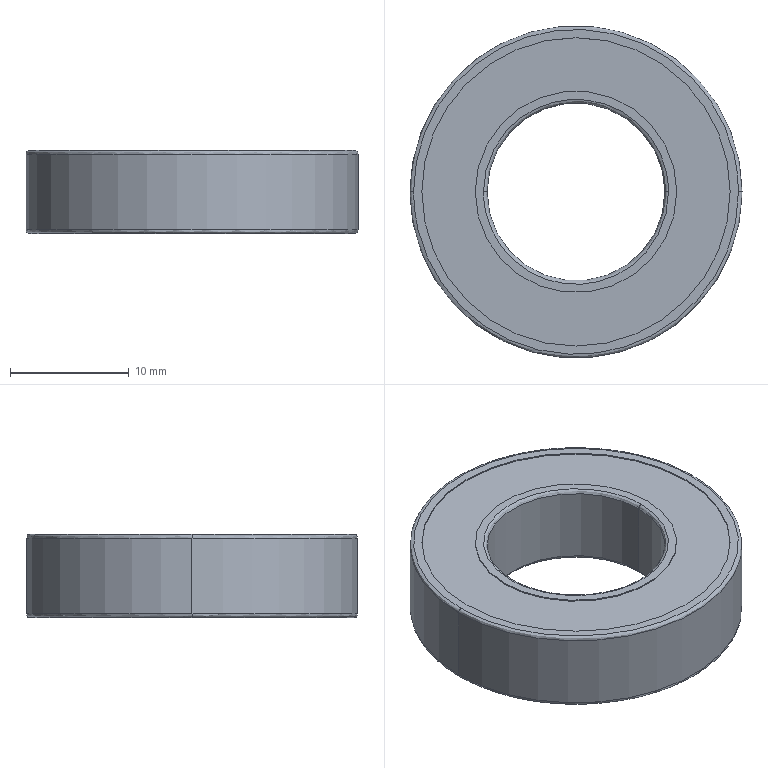Part | SolidWorks | features BaseBody 1 | 1 solid | 26 faces | box 28 x 28 x 7 mm | volume 3008 mm3 | cylinder 12 | spline 8 | plane 6 | commonest cylinder face diameters 17 x4 26 x4 15 x2 28 x2
STEP:
#1=CARTESIAN_POINT('',(-13.7,0.,-7.));
#2=VERTEX_POINT('',#1);
#3=CARTESIAN_POINT('',(13.7,0.,-7.));
#4=VERTEX_POINT('',#3);
#5=CARTESIAN_POINT('',(-13.7,0.,-7.));
#6=CARTESIAN_POINT('',(-13.7,-27.4,-7.));
#7=CARTESIAN_POINT('',(13.7,-27.4,-7.));
#8=CARTESIAN_POINT('',(13.7,0.,-7.));
#9=(BOUNDED_CURVE()B_SPLINE_CURVE(3,(#5,#6,#7,#8),.UNSPECIFIED.,.F.,.F.)B_SPLINE_CURVE_WITH_KNOTS((4,4),(0.,0.5),.UNSPECIFIED.)CURVE()GEOMETRIC_REPRESENTATION_ITEM()RATIONAL_B_SPLINE_CURVE((1.,0.3333,0.3333,1.))REPRESENTATION_ITEM(''));
#10=EDGE_CURVE('',#2,#4,#9,.T.);
#11=ORIENTED_EDGE('',*,*,#10,.T.);
#12=CARTESIAN_POINT('',(14.,0.,-6.7));
#13=VERTEX_POINT('',#12);
#14=CARTESIAN_POINT('',(13.7,0.,-6.7));
#15=DIRECTION('',(0.,-1.,0.));
#16=DIRECTION('',(1.,0.,0.));
#17=AXIS2_PLACEMENT_3D('',#14,#15,#16);
#18=CIRCLE('',#17,0.3);
#19=EDGE_CURVE('',#4,#13,#18,.T.);
#20=ORIENTED_EDGE('',*,*,#19,.T.);
#21=CARTESIAN_POINT('',(-14.,0.,-6.7));
#22=VERTEX_POINT('',#21);
#23=CARTESIAN_POINT('',(0.,0.,-6.7));
#24=DIRECTION('',(0.,0.,1.));
#25=DIRECTION('',(1.,0.,0.));
#26=AXIS2_PLACEMENT_3D('',#23,#24,#25);
#27=CIRCLE('',#26,14.);
#28=EDGE_CURVE('',#22,#13,#27,.T.);
#29=ORIENTED_EDGE('',*,*,#28,.F.);
#30=CARTESIAN_POINT('',(-13.7,0.,-6.7));
#31=DIRECTION('',(0.,1.,0.));
#32=DIRECTION('',(-1.,0.,0.));
#33=AXIS2_PLACEMENT_3D('',#30,#31,#32);
#34=CIRCLE('',#33,0.3);
#35=EDGE_CURVE('',#2,#22,#34,.T.);
#36=ORIENTED_EDGE('',*,*,#35,.F.);
#37=EDGE_LOOP('',(#11,#20,#29,#36));
#38=FACE_OUTER_BOUND('',#37,.T.);
#39=CARTESIAN_POINT('',(13.7,0.,-7.));
#40=CARTESIAN_POINT('',(13.7,-27.4,-7.));
#41=CARTESIAN_POINT('',(-13.7,-27.4,-7.));
#42=CARTESIAN_POINT('',(-13.7,0.,-7.));
#43=CARTESIAN_POINT('',(13.876,0.,-7.));
#44=CARTESIAN_POINT('',(13.876,-27.751,-7.));
#45=CARTESIAN_POINT('',(-13.876,-27.751,-7.));
#46=CARTESIAN_POINT('',(-13.876,0.,-7.));
#47=CARTESIAN_POINT('',(14.,0.,-6.876));
#48=CARTESIAN_POINT('',(14.,-28.,-6.876));
#49=CARTESIAN_POINT('',(-14.,-28.,-6.876));
#50=CARTESIAN_POINT('',(-14.,0.,-6.876));
#51=CARTESIAN_POINT('',(14.,0.,-6.7));
#52=CARTESIAN_POINT('',(14.,-28.,-6.7));
#53=CARTESIAN_POINT('',(-14.,-28.,-6.7));
#54=CARTESIAN_POINT('',(-14.,0.,-6.7));
#55=(BOUNDED_SURFACE()B_SPLINE_SURFACE(3,3,((#39,#40,#41,#42),(#43,#44,#45,#46),(#47,#48,#49,#50),(#51,#52,#53,#54)),.UNSPECIFIED.,.F.,.F.,.F.)B_SPLINE_SURFACE_WITH_KNOTS((4,4),(4,4),(0.,1.),(0.,1.),.UNSPECIFIED.)GEOMETRIC_REPRESENTATION_ITEM()RATIONAL_B_SPLINE_SURFACE(((1.,0.3333,0.3333,1.),(0.8047,0.2682,0.2682,0.8047),(0.8047,0.2682,0.2682,0.8047),(1.,0.3333,0.3333,1.)))REPRESENTATION_ITEM('')SURFACE());
#56=ADVANCED_FACE('',(#38),#55,.T.);
#57=CARTESIAN_POINT('',(14.,0.,-0.3));
#58=VERTEX_POINT('',#57);
#59=CARTESIAN_POINT('',(-14.,0.,-0.3));
#60=VERTEX_POINT('',#59);
#61=CARTESIAN_POINT('',(0.,0.,-0.3));
#62=DIRECTION('',(0.,0.,-1.));
#63=DIRECTION('',(1.,0.,0.));
#64=AXIS2_PLACEMENT_3D('',#61,#62,#63);
#65=CIRCLE('',#64,14.);
#66=EDGE_CURVE('',#58,#60,#65,.T.);
#67=ORIENTED_EDGE('',*,*,#66,.F.);
#68=CARTESIAN_POINT('',(13.7,0.,0.));
#69=VERTEX_POINT('',#68);
#70=CARTESIAN_POINT('',(13.7,0.,-0.3));
#71=DIRECTION('',(0.,-1.,0.));
#72=DIRECTION('',(1.,0.,0.));
#73=AXIS2_PLACEMENT_3D('',#70,#71,#72);
#74=CIRCLE('',#73,0.3);
#75=EDGE_CURVE('',#58,#69,#74,.T.);
#76=ORIENTED_EDGE('',*,*,#75,.T.);
#77=CARTESIAN_POINT('',(-13.7,0.,0.));
#78=VERTEX_POINT('',#77);
#79=CARTESIAN_POINT('',(13.7,0.,0.));
#80=CARTESIAN_POINT('',(13.7,-27.4,0.));
#81=CARTESIAN_POINT('',(-13.7,-27.4,0.));
#82=CARTESIAN_POINT('',(-13.7,0.,0.));
#83=(BOUNDED_CURVE()B_SPLINE_CURVE(3,(#79,#80,#81,#82),.UNSPECIFIED.,.F.,.F.)B_SPLINE_CURVE_WITH_KNOTS((4,4),(0.5,1.),.UNSPECIFIED.)CURVE()GEOMETRIC_REPRESENTATION_ITEM()RATIONAL_B_SPLINE_CURVE((1.,0.3333,0.3333,1.))REPRESENTATION_ITEM(''));
#84=EDGE_CURVE('',#69,#78,#83,.T.);
#85=ORIENTED_EDGE('',*,*,#84,.T.);
#86=CARTESIAN_POINT('',(-13.7,0.,-0.3));
#87=DIRECTION('',(0.,1.,0.));
#88=DIRECTION('',(-1.,0.,0.));
#89=AXIS2_PLACEMENT_3D('',#86,#87,#88);
#90=CIRCLE('',#89,0.3);
#91=EDGE_CURVE('',#60,#78,#90,.T.);
#92=ORIENTED_EDGE('',*,*,#91,.F.);
#93=EDGE_LOOP('',(#67,#76,#85,#92));
#94=FACE_OUTER_BOUND('',#93,.T.);
#95=CARTESIAN_POINT('',(14.,0.,-0.3));
#96=CARTESIAN_POINT('',(14.,-28.,-0.3));
#97=CARTESIAN_POINT('',(-14.,-28.,-0.3));
#98=CARTESIAN_POINT('',(-14.,0.,-0.3));
#99=CARTESIAN_POINT('',(14.,0.,-0.1243));
#100=CARTESIAN_POINT('',(14.,-28.,-0.1243));
#101=CARTESIAN_POINT('',(-14.,-28.,-0.1243));
#102=CARTESIAN_POINT('',(-14.,0.,-0.1243));
#103=CARTESIAN_POINT('',(13.876,0.,0.));
#104=CARTESIAN_POINT('',(13.876,-27.751,0.));
#105=CARTESIAN_POINT('',(-13.876,-27.751,0.));
#106=CARTESIAN_POINT('',(-13.876,0.,0.));
#107=CARTESIAN_POINT('',(13.7,0.,0.));
#108=CARTESIAN_POINT('',(13.7,-27.4,0.));
#109=CARTESIAN_POINT('',(-13.7,-27.4,0.));
#110=CARTESIAN_POINT('',(-13.7,0.,0.));
#111=(BOUNDED_SURFACE()B_SPLINE_SURFACE(3,3,((#95,#96,#97,#98),(#99,#100,#101,#102),(#103,#104,#105,#106),(#107,#108,#109,#110)),.UNSPECIFIED.,.F.,.F.,.F.)B_SPLINE_SURFACE_WITH_KNOTS((4,4),(4,4),(0.,1.),(0.,1.),.UNSPECIFIED.)GEOMETRIC_REPRESENTATION_ITEM()RATIONAL_B_SPLINE_SURFACE(((1.,0.3333,0.3333,1.),(0.8047,0.2682,0.2682,0.8047),(0.8047,0.2682,0.2682,0.8047),(1.,0.3333,0.3333,1.)))REPRESENTATION_ITEM('')SURFACE());
#112=ADVANCED_FACE('',(#94),#111,.T.);
#113=CARTESIAN_POINT('',(-7.5,0.,-6.7));
#114=VERTEX_POINT('',#113);
#115=CARTESIAN_POINT('',(7.5,0.,-6.7));
#116=VERTEX_POINT('',#115);
#117=CARTESIAN_POINT('',(0.,0.,-6.7));
#118=DIRECTION('',(0.,0.,1.));
#119=DIRECTION('',(-1.,0.,0.));
#120=AXIS2_PLACEMENT_3D('',#117,#118,#119);
#121=CIRCLE('',#120,7.5);
#122=EDGE_CURVE('',#114,#116,#121,.T.);
#123=ORIENTED_EDGE('',*,*,#122,.T.);
#124=CARTESIAN_POINT('',(7.8,0.,-7.));
#125=VERTEX_POINT('',#124);
#126=CARTESIAN_POINT('',(7.8,0.,-6.7));
#127=DIRECTION('',(0.,-1.,0.));
#128=DIRECTION('',(1.,0.,0.));
#129=AXIS2_PLACEMENT_3D('',#126,#127,#128);
#130=CIRCLE('',#129,0.3);
#131=EDGE_CURVE('',#116,#125,#130,.T.);
#132=ORIENTED_EDGE('',*,*,#131,.T.);
#133=CARTESIAN_POINT('',(-7.8,0.,-7.));
#134=VERTEX_POINT('',#133);
#135=CARTESIAN_POINT('',(-7.8,0.,-7.));
#136=CARTESIAN_POINT('',(-7.8,-0.2385,-7.));
#137=CARTESIAN_POINT('',(-7.784,-0.5947,-7.));
#138=CARTESIAN_POINT('',(-7.736,-1.008,-7.));
#139=CARTESIAN_POINT('',(-7.705,-1.214,-7.));
#140=CARTESIAN_POINT('',(-7.691,-1.302,-7.));
#141=CARTESIAN_POINT('',(-7.68,-1.361,-7.));
#142=CARTESIAN_POINT('',(-7.676,-1.388,-7.));
#143=CARTESIAN_POINT('',(-7.624,-1.668,-7.));
#144=CARTESIAN_POINT('',(-7.537,-2.036,-7.));
#145=CARTESIAN_POINT('',(-7.405,-2.456,-7.));
#146=CARTESIAN_POINT('',(-7.331,-2.664,-7.));
#147=CARTESIAN_POINT('',(-7.298,-2.753,-7.));
#148=CARTESIAN_POINT('',(-7.275,-2.812,-7.));
#149=CARTESIAN_POINT('',(-7.264,-2.841,-7.));
#150=CARTESIAN_POINT('',(-7.155,-3.116,-7.));
#151=CARTESIAN_POINT('',(-6.992,-3.474,-7.));
#152=CARTESIAN_POINT('',(-6.771,-3.877,-7.));
#153=CARTESIAN_POINT('',(-6.669,-4.046,-7.));
#154=CARTESIAN_POINT('',(-6.6,-4.157,-7.));
#155=CARTESIAN_POINT('',(-6.565,-4.212,-7.));
#156=CARTESIAN_POINT('',(-6.234,-4.719,-7.));
#157=CARTESIAN_POINT('',(-5.896,-5.135,-7.));
#158=CARTESIAN_POINT('',(-5.325,-5.706,-7.));
#159=CARTESIAN_POINT('',(-5.027,-5.975,-7.));
#160=CARTESIAN_POINT('',(-4.655,-6.261,-7.));
#161=CARTESIAN_POINT('',(-4.491,-6.378,-7.));
#162=CARTESIAN_POINT('',(-4.38,-6.454,-7.));
#163=CARTESIAN_POINT('',(-4.323,-6.493,-7.));
#164=CARTESIAN_POINT('',(-4.048,-6.673,-7.));
#165=CARTESIAN_POINT('',(-3.708,-6.871,-7.));
#166=CARTESIAN_POINT('',(-3.295,-7.072,-7.));
#167=CARTESIAN_POINT('',(-3.084,-7.165,-7.));
#168=CARTESIAN_POINT('',(-2.993,-7.203,-7.));
#169=CARTESIAN_POINT('',(-2.932,-7.228,-7.));
#170=CARTESIAN_POINT('',(-2.901,-7.241,-7.));
#171=CARTESIAN_POINT('',(-2.636,-7.345,-7.));
#172=CARTESIAN_POINT('',(-2.278,-7.467,-7.));
#173=CARTESIAN_POINT('',(-1.852,-7.579,-7.));
#174=CARTESIAN_POINT('',(-1.636,-7.627,-7.));
#175=CARTESIAN_POINT('',(-1.543,-7.646,-7.));
#176=CARTESIAN_POINT('',(-1.481,-7.658,-7.));
#177=CARTESIAN_POINT('',(-1.449,-7.664,-7.));
#178=CARTESIAN_POINT('',(-0.9505,-7.757,-7.));
#179=CARTESIAN_POINT('',(-0.4767,-7.8,-7.));
#180=CARTESIAN_POINT('',(0.2384,-7.8,-7.));
#181=CARTESIAN_POINT('',(0.5946,-7.784,-7.));
#182=CARTESIAN_POINT('',(1.008,-7.736,-7.));
#183=CARTESIAN_POINT('',(1.214,-7.705,-7.));
#184=CARTESIAN_POINT('',(1.302,-7.691,-7.));
#185=CARTESIAN_POINT('',(1.361,-7.68,-7.));
#186=CARTESIAN_POINT('',(1.388,-7.676,-7.));
#187=CARTESIAN_POINT('',(1.668,-7.624,-7.));
#188=CARTESIAN_POINT('',(2.036,-7.537,-7.));
#189=CARTESIAN_POINT('',(2.456,-7.405,-7.));
#190=CARTESIAN_POINT('',(2.664,-7.331,-7.));
#191=CARTESIAN_POINT('',(2.753,-7.298,-7.));
#192=CARTESIAN_POINT('',(2.812,-7.275,-7.));
#193=CARTESIAN_POINT('',(2.841,-7.264,-7.));
#194=CARTESIAN_POINT('',(3.116,-7.155,-7.));
#195=CARTESIAN_POINT('',(3.474,-6.992,-7.));
#196=CARTESIAN_POINT('',(3.877,-6.771,-7.));
#197=CARTESIAN_POINT('',(4.046,-6.669,-7.));
#198=CARTESIAN_POINT('',(4.157,-6.6,-7.));
#199=CARTESIAN_POINT('',(4.212,-6.565,-7.));
#200=CARTESIAN_POINT('',(4.719,-6.234,-7.));
#201=CARTESIAN_POINT('',(5.135,-5.896,-7.));
#202=CARTESIAN_POINT('',(5.706,-5.325,-7.));
#203=CARTESIAN_POINT('',(5.975,-5.027,-7.));
#204=CARTESIAN_POINT('',(6.261,-4.655,-7.));
#205=CARTESIAN_POINT('',(6.378,-4.491,-7.));
#206=CARTESIAN_POINT('',(6.454,-4.38,-7.));
#207=CARTESIAN_POINT('',(6.493,-4.323,-7.));
#208=CARTESIAN_POINT('',(6.673,-4.048,-7.));
#209=CARTESIAN_POINT('',(6.871,-3.708,-7.));
#210=CARTESIAN_POINT('',(7.072,-3.295,-7.));
#211=CARTESIAN_POINT('',(7.165,-3.084,-7.));
#212=CARTESIAN_POINT('',(7.203,-2.993,-7.));
#213=CARTESIAN_POINT('',(7.228,-2.932,-7.));
#214=CARTESIAN_POINT('',(7.241,-2.901,-7.));
#215=CARTESIAN_POINT('',(7.345,-2.636,-7.));
#216=CARTESIAN_POINT('',(7.467,-2.278,-7.));
#217=CARTESIAN_POINT('',(7.579,-1.852,-7.));
#218=CARTESIAN_POINT('',(7.627,-1.636,-7.));
#219=CARTESIAN_POINT('',(7.646,-1.543,-7.));
#220=CARTESIAN_POINT('',(7.658,-1.481,-7.));
#221=CARTESIAN_POINT('',(7.664,-1.449,-7.));
#222=CARTESIAN_POINT('',(7.757,-0.9505,-7.));
#223=CARTESIAN_POINT('',(7.8,-0.4767,-7.));
#224=CARTESIAN_POINT('',(7.8,0.,-7.));
#225=B_SPLINE_CURVE_WITH_KNOTS('',3,(#135,#136,#137,#138,#139,#140,#141,#142,#143,#144,#145,#146,#147,#148,#149,#150,#151,#152,#153,#154,#155,#156,#157,#158,#159,#160,#161,#162,#163,#164,#165,#166,#167,#168,#169,#170,#171,#172,#173,#174,#175,#176,#177,#178,#179,#180,#181,#182,#183,#184,#185,#186,#187,#188,#189,#190,#191,#192,#193,#194,#195,#196,#197,#198,#199,#200,#201,#202,#203,#204,#205,#206,#207,#208,#209,#210,#211,#212,#213,#214,#215,#216,#217,#218,#219,#220,#221,#222,#223,#224),.UNSPECIFIED.,.F.,.F.,(4,1,1,1,2,2,1,1,1,2,2,1,1,2,2,2,1,1,2,2,1,1,1,2,2,1,1,1,2,2,2,1,1,1,2,2,1,1,1,2,2,1,1,2,2,2,1,1,2,2,1,1,1,2,2,1,1,1,2,2,4),(0.,0.01562,0.02344,0.02734,0.0293,0.03125,0.04687,0.05469,0.05859,0.06055,0.0625,0.07812,0.08594,0.08984,0.09375,0.125,0.1406,0.1484,0.1523,0.1562,0.1719,0.1797,0.1836,0.1855,0.1875,0.2031,0.2109,0.2148,0.2168,0.2187,0.25,0.2656,0.2734,0.2773,0.2793,0.2812,0.2969,0.3047,0.3086,0.3105,0.3125,0.3281,0.3359,0.3398,0.3437,0.375,0.3906,0.3984,0.4023,0.4062,0.4219,0.4297,0.4336,0.4355,0.4375,0.4531,0.4609,0.4648,0.4668,0.4687,0.5),.UNSPECIFIED.);
#226=EDGE_CURVE('',#134,#125,#225,.T.);
#227=ORIENTED_EDGE('',*,*,#226,.F.);
#228=CARTESIAN_POINT('',(-7.8,0.,-6.7));
#229=DIRECTION('',(0.,1.,0.));
#230=DIRECTION('',(-1.,0.,0.));
#231=AXIS2_PLACEMENT_3D('',#228,#229,#230);
#232=CIRCLE('',#231,0.3);
#233=EDGE_CURVE('',#114,#134,#232,.T.);
#234=ORIENTED_EDGE('',*,*,#233,.F.);
#235=EDGE_LOOP('',(#123,#132,#227,#234));
#236=FACE_OUTER_BOUND('',#235,.T.);
#237=CARTESIAN_POINT('',(7.5,0.,-6.7));
#238=CARTESIAN_POINT('',(7.5,-15.,-6.7));
#239=CARTESIAN_POINT('',(-7.5,-15.,-6.7));
#240=CARTESIAN_POINT('',(-7.5,0.,-6.7));
#241=CARTESIAN_POINT('',(7.5,0.,-6.876));
#242=CARTESIAN_POINT('',(7.5,-15.,-6.876));
#243=CARTESIAN_POINT('',(-7.5,-15.,-6.876));
#244=CARTESIAN_POINT('',(-7.5,0.,-6.876));
#245=CARTESIAN_POINT('',(7.624,0.,-7.));
#246=CARTESIAN_POINT('',(7.624,-15.249,-7.));
#247=CARTESIAN_POINT('',(-7.624,-15.249,-7.));
#248=CARTESIAN_POINT('',(-7.624,0.,-7.));
#249=CARTESIAN_POINT('',(7.8,0.,-7.));
#250=CARTESIAN_POINT('',(7.8,-15.6,-7.));
#251=CARTESIAN_POINT('',(-7.8,-15.6,-7.));
#252=CARTESIAN_POINT('',(-7.8,0.,-7.));
#253=(BOUNDED_SURFACE()B_SPLINE_SURFACE(3,3,((#237,#238,#239,#240),(#241,#242,#243,#244),(#245,#246,#247,#248),(#249,#250,#251,#252)),.UNSPECIFIED.,.F.,.F.,.F.)B_SPLINE_SURFACE_WITH_KNOTS((4,4),(4,4),(0.,1.),(0.,1.),.UNSPECIFIED.)GEOMETRIC_REPRESENTATION_ITEM()RATIONAL_B_SPLINE_SURFACE(((1.,0.3333,0.3333,1.),(0.8047,0.2682,0.2682,0.8047),(0.8047,0.2682,0.2682,0.8047),(1.,0.3333,0.3333,1.)))REPRESENTATION_ITEM('')SURFACE());
#254=ADVANCED_FACE('',(#236),#253,.T.);
#255=CARTESIAN_POINT('',(7.8,0.,0.));
#256=VERTEX_POINT('',#255);
#257=CARTESIAN_POINT('',(-7.8,0.,0.));
#258=VERTEX_POINT('',#257);
#259=CARTESIAN_POINT('',(7.8,0.,0.));
#260=CARTESIAN_POINT('',(7.8,-0.2384,0.));
#261=CARTESIAN_POINT('',(7.784,-0.5946,0.));
#262=CARTESIAN_POINT('',(7.736,-1.008,0.));
#263=CARTESIAN_POINT('',(7.705,-1.214,0.));
#264=CARTESIAN_POINT('',(7.691,-1.302,0.));
#265=CARTESIAN_POINT('',(7.68,-1.361,0.));
#266=CARTESIAN_POINT('',(7.676,-1.388,0.));
#267=CARTESIAN_POINT('',(7.624,-1.668,0.));
#268=CARTESIAN_POINT('',(7.537,-2.036,0.));
#269=CARTESIAN_POINT('',(7.405,-2.456,0.));
#270=CARTESIAN_POINT('',(7.331,-2.664,0.));
#271=CARTESIAN_POINT('',(7.298,-2.753,0.));
#272=CARTESIAN_POINT('',(7.275,-2.812,0.));
#273=CARTESIAN_POINT('',(7.264,-2.841,0.));
#274=CARTESIAN_POINT('',(7.155,-3.116,0.));
#275=CARTESIAN_POINT('',(6.992,-3.474,0.));
#276=CARTESIAN_POINT('',(6.771,-3.877,0.));
#277=CARTESIAN_POINT('',(6.669,-4.046,0.));
#278=CARTESIAN_POINT('',(6.6,-4.157,0.));
#279=CARTESIAN_POINT('',(6.565,-4.212,0.));
#280=CARTESIAN_POINT('',(6.234,-4.719,0.));
#281=CARTESIAN_POINT('',(5.896,-5.135,0.));
#282=CARTESIAN_POINT('',(5.325,-5.706,0.));
#283=CARTESIAN_POINT('',(5.027,-5.975,0.));
#284=CARTESIAN_POINT('',(4.655,-6.261,0.));
#285=CARTESIAN_POINT('',(4.491,-6.378,0.));
#286=CARTESIAN_POINT('',(4.38,-6.454,0.));
#287=CARTESIAN_POINT('',(4.323,-6.493,0.));
#288=CARTESIAN_POINT('',(4.048,-6.673,0.));
#289=CARTESIAN_POINT('',(3.708,-6.871,0.));
#290=CARTESIAN_POINT('',(3.295,-7.072,0.));
#291=CARTESIAN_POINT('',(3.084,-7.165,0.));
#292=CARTESIAN_POINT('',(2.993,-7.203,0.));
#293=CARTESIAN_POINT('',(2.932,-7.228,0.));
#294=CARTESIAN_POINT('',(2.901,-7.241,0.));
#295=CARTESIAN_POINT('',(2.636,-7.345,0.));
#296=CARTESIAN_POINT('',(2.278,-7.467,0.));
#297=CARTESIAN_POINT('',(1.852,-7.579,0.));
#298=CARTESIAN_POINT('',(1.636,-7.627,0.));
#299=CARTESIAN_POINT('',(1.543,-7.646,0.));
#300=CARTESIAN_POINT('',(1.481,-7.658,0.));
#301=CARTESIAN_POINT('',(1.449,-7.664,0.));
#302=CARTESIAN_POINT('',(0.9505,-7.757,0.));
#303=CARTESIAN_POINT('',(0.4767,-7.8,0.));
#304=CARTESIAN_POINT('',(-0.2384,-7.8,0.));
#305=CARTESIAN_POINT('',(-0.5946,-7.784,0.));
#306=CARTESIAN_POINT('',(-1.008,-7.736,0.));
#307=CARTESIAN_POINT('',(-1.214,-7.705,0.));
#308=CARTESIAN_POINT('',(-1.302,-7.691,0.));
#309=CARTESIAN_POINT('',(-1.361,-7.68,0.));
#310=CARTESIAN_POINT('',(-1.388,-7.676,0.));
#311=CARTESIAN_POINT('',(-1.668,-7.624,0.));
#312=CARTESIAN_POINT('',(-2.036,-7.537,0.));
#313=CARTESIAN_POINT('',(-2.456,-7.405,0.));
#314=CARTESIAN_POINT('',(-2.664,-7.331,0.));
#315=CARTESIAN_POINT('',(-2.753,-7.298,0.));
#316=CARTESIAN_POINT('',(-2.812,-7.275,0.));
#317=CARTESIAN_POINT('',(-2.841,-7.264,0.));
#318=CARTESIAN_POINT('',(-3.116,-7.155,0.));
#319=CARTESIAN_POINT('',(-3.474,-6.992,0.));
#320=CARTESIAN_POINT('',(-3.877,-6.771,0.));
#321=CARTESIAN_POINT('',(-4.046,-6.669,0.));
#322=CARTESIAN_POINT('',(-4.157,-6.6,0.));
#323=CARTESIAN_POINT('',(-4.212,-6.565,0.));
#324=CARTESIAN_POINT('',(-4.719,-6.234,0.));
#325=CARTESIAN_POINT('',(-5.135,-5.896,0.));
#326=CARTESIAN_POINT('',(-5.706,-5.325,0.));
#327=CARTESIAN_POINT('',(-5.975,-5.027,0.));
#328=CARTESIAN_POINT('',(-6.261,-4.655,0.));
#329=CARTESIAN_POINT('',(-6.378,-4.491,0.));
#330=CARTESIAN_POINT('',(-6.454,-4.38,0.));
#331=CARTESIAN_POINT('',(-6.493,-4.323,0.));
#332=CARTESIAN_POINT('',(-6.673,-4.048,0.));
#333=CARTESIAN_POINT('',(-6.871,-3.708,0.));
#334=CARTESIAN_POINT('',(-7.072,-3.295,0.));
#335=CARTESIAN_POINT('',(-7.165,-3.084,0.));
#336=CARTESIAN_POINT('',(-7.203,-2.993,0.));
#337=CARTESIAN_POINT('',(-7.228,-2.932,0.));
#338=CARTESIAN_POINT('',(-7.241,-2.901,0.));
#339=CARTESIAN_POINT('',(-7.345,-2.636,0.));
#340=CARTESIAN_POINT('',(-7.467,-2.278,0.));
#341=CARTESIAN_POINT('',(-7.579,-1.852,0.));
#342=CARTESIAN_POINT('',(-7.627,-1.636,0.));
#343=CARTESIAN_POINT('',(-7.646,-1.543,0.));
#344=CARTESIAN_POINT('',(-7.658,-1.481,0.));
#345=CARTESIAN_POINT('',(-7.664,-1.449,0.));
#346=CARTESIAN_POINT('',(-7.757,-0.9504,0.));
#347=CARTESIAN_POINT('',(-7.8,-0.4773,0.));
#348=CARTESIAN_POINT('',(-7.8,0.,0.));
#349=B_SPLINE_CURVE_WITH_KNOTS('',3,(#259,#260,#261,#262,#263,#264,#265,#266,#267,#268,#269,#270,#271,#272,#273,#274,#275,#276,#277,#278,#279,#280,#281,#282,#283,#284,#285,#286,#287,#288,#289,#290,#291,#292,#293,#294,#295,#296,#297,#298,#299,#300,#301,#302,#303,#304,#305,#306,#307,#308,#309,#310,#311,#312,#313,#314,#315,#316,#317,#318,#319,#320,#321,#322,#323,#324,#325,#326,#327,#328,#329,#330,#331,#332,#333,#334,#335,#336,#337,#338,#339,#340,#341,#342,#343,#344,#345,#346,#347,#348),.UNSPECIFIED.,.F.,.F.,(4,1,1,1,2,2,1,1,1,2,2,1,1,2,2,2,1,1,2,2,1,1,1,2,2,1,1,1,2,2,2,1,1,1,2,2,1,1,1,2,2,1,1,2,2,2,1,1,2,2,1,1,1,2,2,1,1,1,2,2,4),(0.5,0.5156,0.5234,0.5273,0.5293,0.5313,0.5469,0.5547,0.5586,0.5605,0.5625,0.5781,0.5859,0.5898,0.5938,0.625,0.6406,0.6484,0.6523,0.6562,0.6719,0.6797,0.6836,0.6855,0.6875,0.7031,0.7109,0.7148,0.7168,0.7187,0.75,0.7656,0.7734,0.7773,0.7793,0.7812,0.7969,0.8047,0.8086,0.8105,0.8125,0.8281,0.8359,0.8398,0.8437,0.875,0.8906,0.8984,0.9023,0.9062,0.9219,0.9297,0.9336,0.9355,0.9375,0.9531,0.9609,0.9648,0.9668,0.9688,1.),.UNSPECIFIED.);
#350=EDGE_CURVE('',#256,#258,#349,.T.);
#351=ORIENTED_EDGE('',*,*,#350,.F.);
#352=CARTESIAN_POINT('',(7.5,0.,-0.3));
#353=VERTEX_POINT('',#352);
#354=CARTESIAN_POINT('',(7.8,0.,-0.3));
#355=DIRECTION('',(0.,-1.,0.));
#356=DIRECTION('',(1.,0.,0.));
#357=AXIS2_PLACEMENT_3D('',#354,#355,#356);
#358=CIRCLE('',#357,0.3);
#359=EDGE_CURVE('',#256,#353,#358,.T.);
#360=ORIENTED_EDGE('',*,*,#359,.T.);
#361=CARTESIAN_POINT('',(-7.5,0.,-0.3));
#362=VERTEX_POINT('',#361);
#363=CARTESIAN_POINT('',(0.,0.,-0.3));
#364=DIRECTION('',(0.,0.,-1.));
#365=DIRECTION('',(-1.,0.,0.));
#366=AXIS2_PLACEMENT_3D('',#363,#364,#365);
#367=CIRCLE('',#366,7.5);
#368=EDGE_CURVE('',#353,#362,#367,.T.);
#369=ORIENTED_EDGE('',*,*,#368,.T.);
#370=CARTESIAN_POINT('',(-7.8,0.,-0.3));
#371=DIRECTION('',(0.,1.,0.));
#372=DIRECTION('',(-1.,0.,0.));
#373=AXIS2_PLACEMENT_3D('',#370,#371,#372);
#374=CIRCLE('',#373,0.3);
#375=EDGE_CURVE('',#258,#362,#374,.T.);
#376=ORIENTED_EDGE('',*,*,#375,.F.);
#377=EDGE_LOOP('',(#351,#360,#369,#376));
#378=FACE_OUTER_BOUND('',#377,.T.);
#379=CARTESIAN_POINT('',(7.8,0.,0.));
#380=CARTESIAN_POINT('',(7.8,-15.6,0.));
#381=CARTESIAN_POINT('',(-7.8,-15.6,0.));
#382=CARTESIAN_POINT('',(-7.8,0.,0.));
#383=CARTESIAN_POINT('',(7.624,0.,0.));
#384=CARTESIAN_POINT('',(7.624,-15.249,0.));
#385=CARTESIAN_POINT('',(-7.624,-15.249,0.));
#386=CARTESIAN_POINT('',(-7.624,0.,0.));
#387=CARTESIAN_POINT('',(7.5,0.,-0.1243));
#388=CARTESIAN_POINT('',(7.5,-15.,-0.1243));
#389=CARTESIAN_POINT('',(-7.5,-15.,-0.1243));
#390=CARTESIAN_POINT('',(-7.5,0.,-0.1243));
#391=CARTESIAN_POINT('',(7.5,0.,-0.3));
#392=CARTESIAN_POINT('',(7.5,-15.,-0.3));
#393=CARTESIAN_POINT('',(-7.5,-15.,-0.3));
#394=CARTESIAN_POINT('',(-7.5,0.,-0.3));
#395=(BOUNDED_SURFACE()B_SPLINE_SURFACE(3,3,((#379,#380,#381,#382),(#383,#384,#385,#386),(#387,#388,#389,#390),(#391,#392,#393,#394)),.UNSPECIFIED.,.F.,.F.,.F.)B_SPLINE_SURFACE_WITH_KNOTS((4,4),(4,4),(0.,1.),(0.,1.),.UNSPECIFIED.)GEOMETRIC_REPRESENTATION_ITEM()RATIONAL_B_SPLINE_SURFACE(((1.,0.3333,0.3333,1.),(0.8047,0.2682,0.2682,0.8047),(0.8047,0.2682,0.2682,0.8047),(1.,0.3333,0.3333,1.)))REPRESENTATION_ITEM('')SURFACE());
#396=ADVANCED_FACE('',(#378),#395,.T.);
#397=CARTESIAN_POINT('',(0.,0.,-6.7));
#398=DIRECTION('',(0.,0.,1.));
#399=DIRECTION('',(1.,0.,0.));
#400=AXIS2_PLACEMENT_3D('',#397,#398,#399);
#401=CIRCLE('',#400,14.);
#402=EDGE_CURVE('',#13,#22,#401,.T.);
#403=ORIENTED_EDGE('',*,*,#402,.T.);
#404=CARTESIAN_POINT('',(-14.,0.,-7.));
#405=DIRECTION('',(0.,0.,1.));
#406=VECTOR('',#405,1000.);
#407=LINE('',#404,#406);
#408=EDGE_CURVE('',#22,#60,#407,.T.);
#409=ORIENTED_EDGE('',*,*,#408,.T.);
#410=CARTESIAN_POINT('',(0.,0.,-0.3));
#411=DIRECTION('',(0.,0.,-1.));
#412=DIRECTION('',(1.,0.,0.));
#413=AXIS2_PLACEMENT_3D('',#410,#411,#412);
#414=CIRCLE('',#413,14.);
#415=EDGE_CURVE('',#60,#58,#414,.T.);
#416=ORIENTED_EDGE('',*,*,#415,.T.);
#417=CARTESIAN_POINT('',(14.,0.,-7.));
#418=DIRECTION('',(0.,0.,1.));
#419=VECTOR('',#418,1000.);
#420=LINE('',#417,#419);
#421=EDGE_CURVE('',#13,#58,#420,.T.);
#422=ORIENTED_EDGE('',*,*,#421,.F.);
#423=EDGE_LOOP('',(#403,#409,#416,#422));
#424=FACE_OUTER_BOUND('',#423,.T.);
#425=CARTESIAN_POINT('',(0.,0.,-7.));
#426=DIRECTION('',(0.,0.,1.));
#427=DIRECTION('',(1.,0.,0.));
#428=AXIS2_PLACEMENT_3D('',#425,#426,#427);
#429=CYLINDRICAL_SURFACE('',#428,14.);
#430=ADVANCED_FACE('',(#424),#429,.T.);
#431=CARTESIAN_POINT('',(-13.,0.,-7.));
#432=VERTEX_POINT('',#431);
#433=CARTESIAN_POINT('',(13.,0.,-7.));
#434=VERTEX_POINT('',#433);
#435=CARTESIAN_POINT('',(0.,0.,-7.));
#436=DIRECTION('',(0.,0.,1.));
#437=DIRECTION('',(1.,0.,0.));
#438=AXIS2_PLACEMENT_3D('',#435,#436,#437);
#439=CIRCLE('',#438,13.);
#440=EDGE_CURVE('',#432,#434,#439,.T.);
#441=ORIENTED_EDGE('',*,*,#440,.F.);
#442=CARTESIAN_POINT('',(-13.,0.,-6.9));
#443=VERTEX_POINT('',#442);
#444=CARTESIAN_POINT('',(-13.,0.,-7.));
#445=DIRECTION('',(0.,0.,1.));
#446=VECTOR('',#445,1000.);
#447=LINE('',#444,#446);
#448=EDGE_CURVE('',#432,#443,#447,.T.);
#449=ORIENTED_EDGE('',*,*,#448,.T.);
#450=CARTESIAN_POINT('',(13.,0.,-6.9));
#451=VERTEX_POINT('',#450);
#452=CARTESIAN_POINT('',(0.,0.,-6.9));
#453=DIRECTION('',(0.,0.,-1.));
#454=DIRECTION('',(1.,0.,0.));
#455=AXIS2_PLACEMENT_3D('',#452,#453,#454);
#456=CIRCLE('',#455,13.);
#457=EDGE_CURVE('',#451,#443,#456,.T.);
#458=ORIENTED_EDGE('',*,*,#457,.F.);
#459=CARTESIAN_POINT('',(13.,0.,-7.));
#460=DIRECTION('',(0.,0.,1.));
#461=VECTOR('',#460,1000.);
#462=LINE('',#459,#461);
#463=EDGE_CURVE('',#434,#451,#462,.T.);
#464=ORIENTED_EDGE('',*,*,#463,.F.);
#465=EDGE_LOOP('',(#441,#449,#458,#464));
#466=FACE_OUTER_BOUND('',#465,.T.);
#467=CARTESIAN_POINT('',(0.,0.,-7.));
#468=DIRECTION('',(0.,0.,1.));
#469=DIRECTION('',(1.,0.,0.));
#470=AXIS2_PLACEMENT_3D('',#467,#468,#469);
#471=CYLINDRICAL_SURFACE('',#470,13.);
#472=ADVANCED_FACE('',(#466),#471,.F.);
#473=CARTESIAN_POINT('',(-13.,0.,-0.1));
#474=VERTEX_POINT('',#473);
#475=CARTESIAN_POINT('',(13.,0.,-0.1));
#476=VERTEX_POINT('',#475);
#477=CARTESIAN_POINT('',(0.,0.,-0.1));
#478=DIRECTION('',(0.,0.,1.));
#479=DIRECTION('',(1.,0.,0.));
#480=AXIS2_PLACEMENT_3D('',#477,#478,#479);
#481=CIRCLE('',#480,13.);
#482=EDGE_CURVE('',#474,#476,#481,.T.);
#483=ORIENTED_EDGE('',*,*,#482,.F.);
#484=CARTESIAN_POINT('',(-13.,0.,0.));
#485=VERTEX_POINT('',#484);
#486=CARTESIAN_POINT('',(-13.,0.,-7.));
#487=DIRECTION('',(0.,0.,1.));
#488=VECTOR('',#487,1000.);
#489=LINE('',#486,#488);
#490=EDGE_CURVE('',#474,#485,#489,.T.);
#491=ORIENTED_EDGE('',*,*,#490,.T.);
#492=CARTESIAN_POINT('',(13.,0.,0.));
#493=VERTEX_POINT('',#492);
#494=CARTESIAN_POINT('',(0.,0.,0.));
#495=DIRECTION('',(0.,0.,-1.));
#496=DIRECTION('',(1.,0.,0.));
#497=AXIS2_PLACEMENT_3D('',#494,#495,#496);
#498=CIRCLE('',#497,13.);
#499=EDGE_CURVE('',#493,#485,#498,.T.);
#500=ORIENTED_EDGE('',*,*,#499,.F.);
#501=CARTESIAN_POINT('',(13.,0.,-7.));
#502=DIRECTION('',(0.,0.,1.));
#503=VECTOR('',#502,1000.);
#504=LINE('',#501,#503);
#505=EDGE_CURVE('',#476,#493,#504,.T.);
#506=ORIENTED_EDGE('',*,*,#505,.F.);
#507=EDGE_LOOP('',(#483,#491,#500,#506));
#508=FACE_OUTER_BOUND('',#507,.T.);
#509=CARTESIAN_POINT('',(0.,0.,-7.));
#510=DIRECTION('',(0.,0.,1.));
#511=DIRECTION('',(1.,0.,0.));
#512=AXIS2_PLACEMENT_3D('',#509,#510,#511);
#513=CYLINDRICAL_SURFACE('',#512,13.);
#514=ADVANCED_FACE('',(#508),#513,.F.);
#515=CARTESIAN_POINT('',(8.5,0.,-7.));
#516=VERTEX_POINT('',#515);
#517=CARTESIAN_POINT('',(-8.5,0.,-7.));
#518=VERTEX_POINT('',#517);
#519=CARTESIAN_POINT('',(0.,0.,-7.));
#520=DIRECTION('',(0.,0.,1.));
#521=DIRECTION('',(1.,0.,0.));
#522=AXIS2_PLACEMENT_3D('',#519,#520,#521);
#523=CIRCLE('',#522,8.5);
#524=EDGE_CURVE('',#516,#518,#523,.T.);
#525=ORIENTED_EDGE('',*,*,#524,.T.);
#526=CARTESIAN_POINT('',(-8.5,0.,-6.9));
#527=VERTEX_POINT('',#526);
#528=CARTESIAN_POINT('',(-8.5,0.,-7.));
#529=DIRECTION('',(0.,0.,1.));
#530=VECTOR('',#529,1000.);
#531=LINE('',#528,#530);
#532=EDGE_CURVE('',#518,#527,#531,.T.);
#533=ORIENTED_EDGE('',*,*,#532,.T.);
#534=CARTESIAN_POINT('',(8.5,0.,-6.9));
#535=VERTEX_POINT('',#534);
#536=CARTESIAN_POINT('',(0.,0.,-6.9));
#537=DIRECTION('',(0.,0.,1.));
#538=DIRECTION('',(1.,0.,0.));
#539=AXIS2_PLACEMENT_3D('',#536,#537,#538);
#540=CIRCLE('',#539,8.5);
#541=EDGE_CURVE('',#535,#527,#540,.T.);
#542=ORIENTED_EDGE('',*,*,#541,.F.);
#543=CARTESIAN_POINT('',(8.5,0.,-7.));
#544=DIRECTION('',(0.,0.,1.));
#545=VECTOR('',#544,1000.);
#546=LINE('',#543,#545);
#547=EDGE_CURVE('',#516,#535,#546,.T.);
#548=ORIENTED_EDGE('',*,*,#547,.F.);
#549=EDGE_LOOP('',(#525,#533,#542,#548));
#550=FACE_OUTER_BOUND('',#549,.T.);
#551=CARTESIAN_POINT('',(0.,0.,-7.));
#552=DIRECTION('',(0.,0.,1.));
#553=DIRECTION('',(1.,0.,0.));
#554=AXIS2_PLACEMENT_3D('',#551,#552,#553);
#555=CYLINDRICAL_SURFACE('',#554,8.5);
#556=ADVANCED_FACE('',(#550),#555,.T.);
#557=CARTESIAN_POINT('',(-8.5,0.,-0.1));
#558=VERTEX_POINT('',#557);
#559=CARTESIAN_POINT('',(8.5,0.,-0.1));
#560=VERTEX_POINT('',#559);
#561=CARTESIAN_POINT('',(0.,0.,-0.1));
#562=DIRECTION('',(0.,0.,-1.));
#563=DIRECTION('',(1.,0.,0.));
#564=AXIS2_PLACEMENT_3D('',#561,#562,#563);
#565=CIRCLE('',#564,8.5);
#566=EDGE_CURVE('',#558,#560,#565,.T.);
#567=ORIENTED_EDGE('',*,*,#566,.F.);
#568=CARTESIAN_POINT('',(-8.5,0.,0.));
#569=VERTEX_POINT('',#568);
#570=CARTESIAN_POINT('',(-8.5,0.,-7.));
#571=DIRECTION('',(0.,0.,1.));
#572=VECTOR('',#571,1000.);
#573=LINE('',#570,#572);
#574=EDGE_CURVE('',#558,#569,#573,.T.);
#575=ORIENTED_EDGE('',*,*,#574,.T.);
#576=CARTESIAN_POINT('',(8.5,0.,0.));
#577=VERTEX_POINT('',#576);
#578=CARTESIAN_POINT('',(0.,0.,0.));
#579=DIRECTION('',(0.,0.,-1.));
#580=DIRECTION('',(1.,0.,0.));
#581=AXIS2_PLACEMENT_3D('',#578,#579,#580);
#582=CIRCLE('',#581,8.5);
#583=EDGE_CURVE('',#569,#577,#582,.T.);
#584=ORIENTED_EDGE('',*,*,#583,.T.);
#585=CARTESIAN_POINT('',(8.5,0.,-7.));
#586=DIRECTION('',(0.,0.,1.));
#587=VECTOR('',#586,1000.);
#588=LINE('',#585,#587);
#589=EDGE_CURVE('',#560,#577,#588,.T.);
#590=ORIENTED_EDGE('',*,*,#589,.F.);
#591=EDGE_LOOP('',(#567,#575,#584,#590));
#592=FACE_OUTER_BOUND('',#591,.T.);
#593=CARTESIAN_POINT('',(0.,0.,-7.));
#594=DIRECTION('',(0.,0.,1.));
#595=DIRECTION('',(1.,0.,0.));
#596=AXIS2_PLACEMENT_3D('',#593,#594,#595);
#597=CYLINDRICAL_SURFACE('',#596,8.5);
#598=ADVANCED_FACE('',(#592),#597,.T.);
#599=ORIENTED_EDGE('',*,*,#122,.F.);
#600=CARTESIAN_POINT('',(-7.5,0.,-7.));
#601=DIRECTION('',(0.,0.,1.));
#602=VECTOR('',#601,1000.);
#603=LINE('',#600,#602);
#604=EDGE_CURVE('',#114,#362,#603,.T.);
#605=ORIENTED_EDGE('',*,*,#604,.T.);
#606=ORIENTED_EDGE('',*,*,#368,.F.);
#607=CARTESIAN_POINT('',(7.5,0.,-7.));
#608=DIRECTION('',(0.,0.,1.));
#609=VECTOR('',#608,1000.);
#610=LINE('',#607,#609);
#611=EDGE_CURVE('',#116,#353,#610,.T.);
#612=ORIENTED_EDGE('',*,*,#611,.F.);
#613=EDGE_LOOP('',(#599,#605,#606,#612));
#614=FACE_OUTER_BOUND('',#613,.T.);
#615=CARTESIAN_POINT('',(0.,0.,-7.));
#616=DIRECTION('',(0.,0.,1.));
#617=DIRECTION('',(1.,0.,0.));
#618=AXIS2_PLACEMENT_3D('',#615,#616,#617);
#619=CYLINDRICAL_SURFACE('',#618,7.5);
#620=ADVANCED_FACE('',(#614),#619,.F.);
#621=ORIENTED_EDGE('',*,*,#408,.F.);
#622=ORIENTED_EDGE('',*,*,#28,.T.);
#623=ORIENTED_EDGE('',*,*,#421,.T.);
#624=ORIENTED_EDGE('',*,*,#66,.T.);
#625=EDGE_LOOP('',(#621,#622,#623,#624));
#626=FACE_OUTER_BOUND('',#625,.T.);
#627=CARTESIAN_POINT('',(0.,0.,-7.));
#628=DIRECTION('',(0.,0.,1.));
#629=DIRECTION('',(1.,0.,0.));
#630=AXIS2_PLACEMENT_3D('',#627,#628,#629);
#631=CYLINDRICAL_SURFACE('',#630,14.);
#632=ADVANCED_FACE('',(#626),#631,.T.);
#633=ORIENTED_EDGE('',*,*,#19,.F.);
#634=CARTESIAN_POINT('',(13.7,0.,-7.));
#635=CARTESIAN_POINT('',(13.7,27.4,-7.));
#636=CARTESIAN_POINT('',(-13.7,27.4,-7.));
#637=CARTESIAN_POINT('',(-13.7,0.,-7.));
#638=(BOUNDED_CURVE()B_SPLINE_CURVE(3,(#634,#635,#636,#637),.UNSPECIFIED.,.F.,.F.)B_SPLINE_CURVE_WITH_KNOTS((4,4),(0.5,1.),.UNSPECIFIED.)CURVE()GEOMETRIC_REPRESENTATION_ITEM()RATIONAL_B_SPLINE_CURVE((1.,0.3333,0.3333,1.))REPRESENTATION_ITEM(''));
#639=EDGE_CURVE('',#4,#2,#638,.T.);
#640=ORIENTED_EDGE('',*,*,#639,.T.);
#641=ORIENTED_EDGE('',*,*,#35,.T.);
#642=ORIENTED_EDGE('',*,*,#402,.F.);
#643=EDGE_LOOP('',(#633,#640,#641,#642));
#644=FACE_OUTER_BOUND('',#643,.T.);
#645=CARTESIAN_POINT('',(-13.7,0.,-7.));
#646=CARTESIAN_POINT('',(-13.7,27.4,-7.));
#647=CARTESIAN_POINT('',(13.7,27.4,-7.));
#648=CARTESIAN_POINT('',(13.7,0.,-7.));
#649=CARTESIAN_POINT('',(-13.876,0.,-7.));
#650=CARTESIAN_POINT('',(-13.876,27.751,-7.));
#651=CARTESIAN_POINT('',(13.876,27.751,-7.));
#652=CARTESIAN_POINT('',(13.876,0.,-7.));
#653=CARTESIAN_POINT('',(-14.,0.,-6.876));
#654=CARTESIAN_POINT('',(-14.,28.,-6.876));
#655=CARTESIAN_POINT('',(14.,28.,-6.876));
#656=CARTESIAN_POINT('',(14.,0.,-6.876));
#657=CARTESIAN_POINT('',(-14.,0.,-6.7));
#658=CARTESIAN_POINT('',(-14.,28.,-6.7));
#659=CARTESIAN_POINT('',(14.,28.,-6.7));
#660=CARTESIAN_POINT('',(14.,0.,-6.7));
#661=(BOUNDED_SURFACE()B_SPLINE_SURFACE(3,3,((#645,#646,#647,#648),(#649,#650,#651,#652),(#653,#654,#655,#656),(#657,#658,#659,#660)),.UNSPECIFIED.,.F.,.F.,.F.)B_SPLINE_SURFACE_WITH_KNOTS((4,4),(4,4),(0.,1.),(0.,1.),.UNSPECIFIED.)GEOMETRIC_REPRESENTATION_ITEM()RATIONAL_B_SPLINE_SURFACE(((1.,0.3333,0.3333,1.),(0.8047,0.2682,0.2682,0.8047),(0.8047,0.2682,0.2682,0.8047),(1.,0.3333,0.3333,1.)))REPRESENTATION_ITEM('')SURFACE());
#662=ADVANCED_FACE('',(#644),#661,.T.);
#663=ORIENTED_EDGE('',*,*,#75,.F.);
#664=ORIENTED_EDGE('',*,*,#415,.F.);
#665=ORIENTED_EDGE('',*,*,#91,.T.);
#666=CARTESIAN_POINT('',(-13.7,0.,0.));
#667=CARTESIAN_POINT('',(-13.7,27.4,0.));
#668=CARTESIAN_POINT('',(13.7,27.4,0.));
#669=CARTESIAN_POINT('',(13.7,0.,0.));
#670=(BOUNDED_CURVE()B_SPLINE_CURVE(3,(#666,#667,#668,#669),.UNSPECIFIED.,.F.,.F.)B_SPLINE_CURVE_WITH_KNOTS((4,4),(0.,0.5),.UNSPECIFIED.)CURVE()GEOMETRIC_REPRESENTATION_ITEM()RATIONAL_B_SPLINE_CURVE((1.,0.3333,0.3333,1.))REPRESENTATION_ITEM(''));
#671=EDGE_CURVE('',#78,#69,#670,.T.);
#672=ORIENTED_EDGE('',*,*,#671,.T.);
#673=EDGE_LOOP('',(#663,#664,#665,#672));
#674=FACE_OUTER_BOUND('',#673,.T.);
#675=CARTESIAN_POINT('',(-14.,0.,-0.3));
#676=CARTESIAN_POINT('',(-14.,28.,-0.3));
#677=CARTESIAN_POINT('',(14.,28.,-0.3));
#678=CARTESIAN_POINT('',(14.,0.,-0.3));
#679=CARTESIAN_POINT('',(-14.,0.,-0.1243));
#680=CARTESIAN_POINT('',(-14.,28.,-0.1243));
#681=CARTESIAN_POINT('',(14.,28.,-0.1243));
#682=CARTESIAN_POINT('',(14.,0.,-0.1243));
#683=CARTESIAN_POINT('',(-13.876,0.,0.));
#684=CARTESIAN_POINT('',(-13.876,27.751,0.));
#685=CARTESIAN_POINT('',(13.876,27.751,0.));
#686=CARTESIAN_POINT('',(13.876,0.,0.));
#687=CARTESIAN_POINT('',(-13.7,0.,0.));
#688=CARTESIAN_POINT('',(-13.7,27.4,0.));
#689=CARTESIAN_POINT('',(13.7,27.4,0.));
#690=CARTESIAN_POINT('',(13.7,0.,0.));
#691=(BOUNDED_SURFACE()B_SPLINE_SURFACE(3,3,((#675,#676,#677,#678),(#679,#680,#681,#682),(#683,#684,#685,#686),(#687,#688,#689,#690)),.UNSPECIFIED.,.F.,.F.,.F.)B_SPLINE_SURFACE_WITH_KNOTS((4,4),(4,4),(0.,1.),(0.,1.),.UNSPECIFIED.)GEOMETRIC_REPRESENTATION_ITEM()RATIONAL_B_SPLINE_SURFACE(((1.,0.3333,0.3333,1.),(0.8047,0.2682,0.2682,0.8047),(0.8047,0.2682,0.2682,0.8047),(1.,0.3333,0.3333,1.)))REPRESENTATION_ITEM('')SURFACE());
#692=ADVANCED_FACE('',(#674),#691,.T.);
#693=CARTESIAN_POINT('',(0.,0.,-7.));
#694=DIRECTION('',(0.,0.,1.));
#695=DIRECTION('',(1.,0.,0.));
#696=AXIS2_PLACEMENT_3D('',#693,#694,#695);
#697=CIRCLE('',#696,13.);
#698=EDGE_CURVE('',#434,#432,#697,.T.);
#699=ORIENTED_EDGE('',*,*,#698,.T.);
#700=ORIENTED_EDGE('',*,*,#440,.T.);
#701=EDGE_LOOP('',(#699,#700));
#702=FACE_BOUND('',#701,.T.);
#703=ORIENTED_EDGE('',*,*,#10,.F.);
#704=ORIENTED_EDGE('',*,*,#639,.F.);
#705=EDGE_LOOP('',(#703,#704));
#706=FACE_OUTER_BOUND('',#705,.T.);
#707=CARTESIAN_POINT('',(0.,13.,-7.));
#708=DIRECTION('',(0.,0.,-1.));
#709=DIRECTION('',(-1.,0.,0.));
#710=AXIS2_PLACEMENT_3D('',#707,#708,#709);
#711=PLANE('',#710);
#712=ADVANCED_FACE('',(#702,#706),#711,.T.);
#713=ORIENTED_EDGE('',*,*,#671,.F.);
#714=ORIENTED_EDGE('',*,*,#84,.F.);
#715=EDGE_LOOP('',(#713,#714));
#716=FACE_OUTER_BOUND('',#715,.T.);
#717=ORIENTED_EDGE('',*,*,#499,.T.);
#718=CARTESIAN_POINT('',(0.,0.,0.));
#719=DIRECTION('',(0.,0.,-1.));
#720=DIRECTION('',(1.,0.,0.));
#721=AXIS2_PLACEMENT_3D('',#718,#719,#720);
#722=CIRCLE('',#721,13.);
#723=EDGE_CURVE('',#485,#493,#722,.T.);
#724=ORIENTED_EDGE('',*,*,#723,.T.);
#725=EDGE_LOOP('',(#717,#724));
#726=FACE_BOUND('',#725,.T.);
#727=CARTESIAN_POINT('',(0.,13.7,0.));
#728=DIRECTION('',(0.,0.,1.));
#729=DIRECTION('',(1.,0.,0.));
#730=AXIS2_PLACEMENT_3D('',#727,#728,#729);
#731=PLANE('',#730);
#732=ADVANCED_FACE('',(#716,#726),#731,.T.);
#733=ORIENTED_EDGE('',*,*,#448,.F.);
#734=ORIENTED_EDGE('',*,*,#698,.F.);
#735=ORIENTED_EDGE('',*,*,#463,.T.);
#736=CARTESIAN_POINT('',(0.,0.,-6.9));
#737=DIRECTION('',(0.,0.,-1.));
#738=DIRECTION('',(1.,0.,0.));
#739=AXIS2_PLACEMENT_3D('',#736,#737,#738);
#740=CIRCLE('',#739,13.);
#741=EDGE_CURVE('',#443,#451,#740,.T.);
#742=ORIENTED_EDGE('',*,*,#741,.F.);
#743=EDGE_LOOP('',(#733,#734,#735,#742));
#744=FACE_OUTER_BOUND('',#743,.T.);
#745=CARTESIAN_POINT('',(0.,0.,-7.));
#746=DIRECTION('',(0.,0.,1.));
#747=DIRECTION('',(1.,0.,0.));
#748=AXIS2_PLACEMENT_3D('',#745,#746,#747);
#749=CYLINDRICAL_SURFACE('',#748,13.);
#750=ADVANCED_FACE('',(#744),#749,.F.);
#751=ORIENTED_EDGE('',*,*,#490,.F.);
#752=CARTESIAN_POINT('',(0.,0.,-0.1));
#753=DIRECTION('',(0.,0.,1.));
#754=DIRECTION('',(1.,0.,0.));
#755=AXIS2_PLACEMENT_3D('',#752,#753,#754);
#756=CIRCLE('',#755,13.);
#757=EDGE_CURVE('',#476,#474,#756,.T.);
#758=ORIENTED_EDGE('',*,*,#757,.F.);
#759=ORIENTED_EDGE('',*,*,#505,.T.);
#760=ORIENTED_EDGE('',*,*,#723,.F.);
#761=EDGE_LOOP('',(#751,#758,#759,#760));
#762=FACE_OUTER_BOUND('',#761,.T.);
#763=CARTESIAN_POINT('',(0.,0.,-7.));
#764=DIRECTION('',(0.,0.,1.));
#765=DIRECTION('',(1.,0.,0.));
#766=AXIS2_PLACEMENT_3D('',#763,#764,#765);
#767=CYLINDRICAL_SURFACE('',#766,13.);
#768=ADVANCED_FACE('',(#762),#767,.F.);
#769=ORIENTED_EDGE('',*,*,#541,.T.);
#770=CARTESIAN_POINT('',(0.,0.,-6.9));
#771=DIRECTION('',(0.,0.,1.));
#772=DIRECTION('',(1.,0.,0.));
#773=AXIS2_PLACEMENT_3D('',#770,#771,#772);
#774=CIRCLE('',#773,8.5);
#775=EDGE_CURVE('',#527,#535,#774,.T.);
#776=ORIENTED_EDGE('',*,*,#775,.T.);
#777=EDGE_LOOP('',(#769,#776));
#778=FACE_BOUND('',#777,.T.);
#779=ORIENTED_EDGE('',*,*,#457,.T.);
#780=ORIENTED_EDGE('',*,*,#741,.T.);
#781=EDGE_LOOP('',(#779,#780));
#782=FACE_OUTER_BOUND('',#781,.T.);
#783=CARTESIAN_POINT('',(0.,8.5,-6.9));
#784=DIRECTION('',(0.,0.,-1.));
#785=DIRECTION('',(-1.,0.,0.));
#786=AXIS2_PLACEMENT_3D('',#783,#784,#785);
#787=PLANE('',#786);
#788=ADVANCED_FACE('',(#778,#782),#787,.T.);
#789=ORIENTED_EDGE('',*,*,#757,.T.);
#790=ORIENTED_EDGE('',*,*,#482,.T.);
#791=EDGE_LOOP('',(#789,#790));
#792=FACE_OUTER_BOUND('',#791,.T.);
#793=CARTESIAN_POINT('',(0.,0.,-0.1));
#794=DIRECTION('',(0.,0.,-1.));
#795=DIRECTION('',(1.,0.,0.));
#796=AXIS2_PLACEMENT_3D('',#793,#794,#795);
#797=CIRCLE('',#796,8.5);
#798=EDGE_CURVE('',#560,#558,#797,.T.);
#799=ORIENTED_EDGE('',*,*,#798,.T.);
#800=ORIENTED_EDGE('',*,*,#566,.T.);
#801=EDGE_LOOP('',(#799,#800));
#802=FACE_BOUND('',#801,.T.);
#803=CARTESIAN_POINT('',(0.,13.,-0.1));
#804=DIRECTION('',(0.,0.,1.));
#805=DIRECTION('',(1.,0.,0.));
#806=AXIS2_PLACEMENT_3D('',#803,#804,#805);
#807=PLANE('',#806);
#808=ADVANCED_FACE('',(#792,#802),#807,.T.);
#809=ORIENTED_EDGE('',*,*,#532,.F.);
#810=CARTESIAN_POINT('',(0.,0.,-7.));
#811=DIRECTION('',(0.,0.,1.));
#812=DIRECTION('',(1.,0.,0.));
#813=AXIS2_PLACEMENT_3D('',#810,#811,#812);
#814=CIRCLE('',#813,8.5);
#815=EDGE_CURVE('',#518,#516,#814,.T.);
#816=ORIENTED_EDGE('',*,*,#815,.T.);
#817=ORIENTED_EDGE('',*,*,#547,.T.);
#818=ORIENTED_EDGE('',*,*,#775,.F.);
#819=EDGE_LOOP('',(#809,#816,#817,#818));
#820=FACE_OUTER_BOUND('',#819,.T.);
#821=CARTESIAN_POINT('',(0.,0.,-7.));
#822=DIRECTION('',(0.,0.,1.));
#823=DIRECTION('',(1.,0.,0.));
#824=AXIS2_PLACEMENT_3D('',#821,#822,#823);
#825=CYLINDRICAL_SURFACE('',#824,8.5);
#826=ADVANCED_FACE('',(#820),#825,.T.);
#827=ORIENTED_EDGE('',*,*,#574,.F.);
#828=ORIENTED_EDGE('',*,*,#798,.F.);
#829=ORIENTED_EDGE('',*,*,#589,.T.);
#830=CARTESIAN_POINT('',(0.,0.,0.));
#831=DIRECTION('',(0.,0.,-1.));
#832=DIRECTION('',(1.,0.,0.));
#833=AXIS2_PLACEMENT_3D('',#830,#831,#832);
#834=CIRCLE('',#833,8.5);
#835=EDGE_CURVE('',#577,#569,#834,.T.);
#836=ORIENTED_EDGE('',*,*,#835,.T.);
#837=EDGE_LOOP('',(#827,#828,#829,#836));
#838=FACE_OUTER_BOUND('',#837,.T.);
#839=CARTESIAN_POINT('',(0.,0.,-7.));
#840=DIRECTION('',(0.,0.,1.));
#841=DIRECTION('',(1.,0.,0.));
#842=AXIS2_PLACEMENT_3D('',#839,#840,#841);
#843=CYLINDRICAL_SURFACE('',#842,8.5);
#844=ADVANCED_FACE('',(#838),#843,.T.);
#845=ORIENTED_EDGE('',*,*,#226,.T.);
#846=CARTESIAN_POINT('',(7.8,0.,-7.));
#847=CARTESIAN_POINT('',(7.8,0.2384,-7.));
#848=CARTESIAN_POINT('',(7.784,0.5946,-7.));
#849=CARTESIAN_POINT('',(7.736,1.008,-7.));
#850=CARTESIAN_POINT('',(7.705,1.214,-7.));
#851=CARTESIAN_POINT('',(7.691,1.302,-7.));
#852=CARTESIAN_POINT('',(7.68,1.361,-7.));
#853=CARTESIAN_POINT('',(7.676,1.388,-7.));
#854=CARTESIAN_POINT('',(7.624,1.668,-7.));
#855=CARTESIAN_POINT('',(7.537,2.036,-7.));
#856=CARTESIAN_POINT('',(7.405,2.456,-7.));
#857=CARTESIAN_POINT('',(7.331,2.664,-7.));
#858=CARTESIAN_POINT('',(7.298,2.753,-7.));
#859=CARTESIAN_POINT('',(7.275,2.812,-7.));
#860=CARTESIAN_POINT('',(7.264,2.841,-7.));
#861=CARTESIAN_POINT('',(7.155,3.116,-7.));
#862=CARTESIAN_POINT('',(6.992,3.474,-7.));
#863=CARTESIAN_POINT('',(6.771,3.877,-7.));
#864=CARTESIAN_POINT('',(6.669,4.046,-7.));
#865=CARTESIAN_POINT('',(6.6,4.157,-7.));
#866=CARTESIAN_POINT('',(6.565,4.212,-7.));
#867=CARTESIAN_POINT('',(6.234,4.719,-7.));
#868=CARTESIAN_POINT('',(5.896,5.135,-7.));
#869=CARTESIAN_POINT('',(5.325,5.706,-7.));
#870=CARTESIAN_POINT('',(5.027,5.975,-7.));
#871=CARTESIAN_POINT('',(4.655,6.261,-7.));
#872=CARTESIAN_POINT('',(4.491,6.378,-7.));
#873=CARTESIAN_POINT('',(4.38,6.454,-7.));
#874=CARTESIAN_POINT('',(4.323,6.493,-7.));
#875=CARTESIAN_POINT('',(4.048,6.673,-7.));
#876=CARTESIAN_POINT('',(3.708,6.871,-7.));
#877=CARTESIAN_POINT('',(3.295,7.072,-7.));
#878=CARTESIAN_POINT('',(3.084,7.165,-7.));
#879=CARTESIAN_POINT('',(2.993,7.203,-7.));
#880=CARTESIAN_POINT('',(2.932,7.228,-7.));
#881=CARTESIAN_POINT('',(2.901,7.241,-7.));
#882=CARTESIAN_POINT('',(2.636,7.345,-7.));
#883=CARTESIAN_POINT('',(2.278,7.467,-7.));
#884=CARTESIAN_POINT('',(1.852,7.579,-7.));
#885=CARTESIAN_POINT('',(1.636,7.627,-7.));
#886=CARTESIAN_POINT('',(1.543,7.646,-7.));
#887=CARTESIAN_POINT('',(1.481,7.658,-7.));
#888=CARTESIAN_POINT('',(1.449,7.664,-7.));
#889=CARTESIAN_POINT('',(0.9505,7.757,-7.));
#890=CARTESIAN_POINT('',(0.4767,7.8,-7.));
#891=CARTESIAN_POINT('',(-0.2384,7.8,-7.));
#892=CARTESIAN_POINT('',(-0.5946,7.784,-7.));
#893=CARTESIAN_POINT('',(-1.008,7.736,-7.));
#894=CARTESIAN_POINT('',(-1.214,7.705,-7.));
#895=CARTESIAN_POINT('',(-1.302,7.691,-7.));
#896=CARTESIAN_POINT('',(-1.361,7.68,-7.));
#897=CARTESIAN_POINT('',(-1.388,7.676,-7.));
#898=CARTESIAN_POINT('',(-1.668,7.624,-7.));
#899=CARTESIAN_POINT('',(-2.036,7.537,-7.));
#900=CARTESIAN_POINT('',(-2.456,7.405,-7.));
#901=CARTESIAN_POINT('',(-2.664,7.331,-7.));
#902=CARTESIAN_POINT('',(-2.753,7.298,-7.));
#903=CARTESIAN_POINT('',(-2.812,7.275,-7.));
#904=CARTESIAN_POINT('',(-2.841,7.264,-7.));
#905=CARTESIAN_POINT('',(-3.116,7.155,-7.));
#906=CARTESIAN_POINT('',(-3.474,6.992,-7.));
#907=CARTESIAN_POINT('',(-3.877,6.771,-7.));
#908=CARTESIAN_POINT('',(-4.046,6.669,-7.));
#909=CARTESIAN_POINT('',(-4.157,6.6,-7.));
#910=CARTESIAN_POINT('',(-4.212,6.565,-7.));
#911=CARTESIAN_POINT('',(-4.719,6.234,-7.));
#912=CARTESIAN_POINT('',(-5.135,5.896,-7.));
#913=CARTESIAN_POINT('',(-5.706,5.325,-7.));
#914=CARTESIAN_POINT('',(-5.975,5.027,-7.));
#915=CARTESIAN_POINT('',(-6.261,4.655,-7.));
#916=CARTESIAN_POINT('',(-6.378,4.491,-7.));
#917=CARTESIAN_POINT('',(-6.454,4.38,-7.));
#918=CARTESIAN_POINT('',(-6.493,4.323,-7.));
#919=CARTESIAN_POINT('',(-6.673,4.048,-7.));
#920=CARTESIAN_POINT('',(-6.871,3.708,-7.));
#921=CARTESIAN_POINT('',(-7.072,3.295,-7.));
#922=CARTESIAN_POINT('',(-7.165,3.084,-7.));
#923=CARTESIAN_POINT('',(-7.203,2.993,-7.));
#924=CARTESIAN_POINT('',(-7.228,2.932,-7.));
#925=CARTESIAN_POINT('',(-7.241,2.901,-7.));
#926=CARTESIAN_POINT('',(-7.345,2.636,-7.));
#927=CARTESIAN_POINT('',(-7.467,2.278,-7.));
#928=CARTESIAN_POINT('',(-7.579,1.852,-7.));
#929=CARTESIAN_POINT('',(-7.627,1.636,-7.));
#930=CARTESIAN_POINT('',(-7.646,1.543,-7.));
#931=CARTESIAN_POINT('',(-7.658,1.481,-7.));
#932=CARTESIAN_POINT('',(-7.664,1.449,-7.));
#933=CARTESIAN_POINT('',(-7.757,0.9504,-7.));
#934=CARTESIAN_POINT('',(-7.8,0.4773,-7.));
#935=CARTESIAN_POINT('',(-7.8,0.,-7.));
#936=B_SPLINE_CURVE_WITH_KNOTS('',3,(#846,#847,#848,#849,#850,#851,#852,#853,#854,#855,#856,#857,#858,#859,#860,#861,#862,#863,#864,#865,#866,#867,#868,#869,#870,#871,#872,#873,#874,#875,#876,#877,#878,#879,#880,#881,#882,#883,#884,#885,#886,#887,#888,#889,#890,#891,#892,#893,#894,#895,#896,#897,#898,#899,#900,#901,#902,#903,#904,#905,#906,#907,#908,#909,#910,#911,#912,#913,#914,#915,#916,#917,#918,#919,#920,#921,#922,#923,#924,#925,#926,#927,#928,#929,#930,#931,#932,#933,#934,#935),.UNSPECIFIED.,.F.,.F.,(4,1,1,1,2,2,1,1,1,2,2,1,1,2,2,2,1,1,2,2,1,1,1,2,2,1,1,1,2,2,2,1,1,1,2,2,1,1,1,2,2,1,1,2,2,2,1,1,2,2,1,1,1,2,2,1,1,1,2,2,4),(0.5,0.5156,0.5234,0.5273,0.5293,0.5313,0.5469,0.5547,0.5586,0.5605,0.5625,0.5781,0.5859,0.5898,0.5938,0.625,0.6406,0.6484,0.6523,0.6563,0.6719,0.6797,0.6836,0.6855,0.6875,0.7031,0.7109,0.7148,0.7168,0.7188,0.75,0.7656,0.7734,0.7773,0.7793,0.7813,0.7969,0.8047,0.8086,0.8105,0.8125,0.8281,0.8359,0.8398,0.8438,0.875,0.8906,0.8984,0.9023,0.9063,0.9219,0.9297,0.9336,0.9355,0.9375,0.9531,0.9609,0.9648,0.9668,0.9688,1.),.UNSPECIFIED.);
#937=EDGE_CURVE('',#125,#134,#936,.T.);
#938=ORIENTED_EDGE('',*,*,#937,.T.);
#939=EDGE_LOOP('',(#845,#938));
#940=FACE_BOUND('',#939,.T.);
#941=ORIENTED_EDGE('',*,*,#524,.F.);
#942=ORIENTED_EDGE('',*,*,#815,.F.);
#943=EDGE_LOOP('',(#941,#942));
#944=FACE_OUTER_BOUND('',#943,.T.);
#945=CARTESIAN_POINT('',(0.,7.8,-7.));
#946=DIRECTION('',(0.,0.,-1.));
#947=DIRECTION('',(-1.,0.,0.));
#948=AXIS2_PLACEMENT_3D('',#945,#946,#947);
#949=PLANE('',#948);
#950=ADVANCED_FACE('',(#940,#944),#949,.T.);
#951=ORIENTED_EDGE('',*,*,#835,.F.);
#952=ORIENTED_EDGE('',*,*,#583,.F.);
#953=EDGE_LOOP('',(#951,#952));
#954=FACE_OUTER_BOUND('',#953,.T.);
#955=CARTESIAN_POINT('',(-7.8,0.,0.));
#956=CARTESIAN_POINT('',(-7.8,0.2385,0.));
#957=CARTESIAN_POINT('',(-7.784,0.5947,0.));
#958=CARTESIAN_POINT('',(-7.736,1.008,0.));
#959=CARTESIAN_POINT('',(-7.705,1.214,0.));
#960=CARTESIAN_POINT('',(-7.691,1.302,0.));
#961=CARTESIAN_POINT('',(-7.68,1.361,0.));
#962=CARTESIAN_POINT('',(-7.676,1.388,0.));
#963=CARTESIAN_POINT('',(-7.624,1.668,0.));
#964=CARTESIAN_POINT('',(-7.537,2.036,0.));
#965=CARTESIAN_POINT('',(-7.405,2.456,0.));
#966=CARTESIAN_POINT('',(-7.331,2.664,0.));
#967=CARTESIAN_POINT('',(-7.298,2.753,0.));
#968=CARTESIAN_POINT('',(-7.275,2.812,0.));
#969=CARTESIAN_POINT('',(-7.264,2.841,0.));
#970=CARTESIAN_POINT('',(-7.155,3.116,0.));
#971=CARTESIAN_POINT('',(-6.992,3.474,0.));
#972=CARTESIAN_POINT('',(-6.771,3.877,0.));
#973=CARTESIAN_POINT('',(-6.669,4.046,0.));
#974=CARTESIAN_POINT('',(-6.6,4.157,0.));
#975=CARTESIAN_POINT('',(-6.565,4.212,0.));
#976=CARTESIAN_POINT('',(-6.234,4.719,0.));
#977=CARTESIAN_POINT('',(-5.896,5.135,0.));
#978=CARTESIAN_POINT('',(-5.325,5.706,0.));
#979=CARTESIAN_POINT('',(-5.027,5.975,0.));
#980=CARTESIAN_POINT('',(-4.655,6.261,0.));
#981=CARTESIAN_POINT('',(-4.491,6.378,0.));
#982=CARTESIAN_POINT('',(-4.38,6.454,0.));
#983=CARTESIAN_POINT('',(-4.323,6.493,0.));
#984=CARTESIAN_POINT('',(-4.048,6.673,0.));
#985=CARTESIAN_POINT('',(-3.708,6.871,0.));
#986=CARTESIAN_POINT('',(-3.295,7.072,0.));
#987=CARTESIAN_POINT('',(-3.084,7.165,0.));
#988=CARTESIAN_POINT('',(-2.993,7.203,0.));
#989=CARTESIAN_POINT('',(-2.932,7.228,0.));
#990=CARTESIAN_POINT('',(-2.901,7.241,0.));
#991=CARTESIAN_POINT('',(-2.636,7.345,0.));
#992=CARTESIAN_POINT('',(-2.278,7.467,0.));
#993=CARTESIAN_POINT('',(-1.852,7.579,0.));
#994=CARTESIAN_POINT('',(-1.636,7.627,0.));
#995=CARTESIAN_POINT('',(-1.543,7.646,0.));
#996=CARTESIAN_POINT('',(-1.481,7.658,0.));
#997=CARTESIAN_POINT('',(-1.449,7.664,0.));
#998=CARTESIAN_POINT('',(-0.9505,7.757,0.));
#999=CARTESIAN_POINT('',(-0.4767,7.8,0.));
#1000=CARTESIAN_POINT('',(0.2384,7.8,0.));
#1001=CARTESIAN_POINT('',(0.5946,7.784,0.));
#1002=CARTESIAN_POINT('',(1.008,7.736,0.));
#1003=CARTESIAN_POINT('',(1.214,7.705,0.));
#1004=CARTESIAN_POINT('',(1.302,7.691,0.));
#1005=CARTESIAN_POINT('',(1.361,7.68,0.));
#1006=CARTESIAN_POINT('',(1.388,7.676,0.));
#1007=CARTESIAN_POINT('',(1.668,7.624,0.));
#1008=CARTESIAN_POINT('',(2.036,7.537,0.));
#1009=CARTESIAN_POINT('',(2.456,7.405,0.));
#1010=CARTESIAN_POINT('',(2.664,7.331,0.));
#1011=CARTESIAN_POINT('',(2.753,7.298,0.));
#1012=CARTESIAN_POINT('',(2.812,7.275,0.));
#1013=CARTESIAN_POINT('',(2.841,7.264,0.));
#1014=CARTESIAN_POINT('',(3.116,7.155,0.));
#1015=CARTESIAN_POINT('',(3.474,6.992,0.));
#1016=CARTESIAN_POINT('',(3.877,6.771,0.));
#1017=CARTESIAN_POINT('',(4.046,6.669,0.));
#1018=CARTESIAN_POINT('',(4.157,6.6,0.));
#1019=CARTESIAN_POINT('',(4.212,6.565,0.));
#1020=CARTESIAN_POINT('',(4.719,6.234,0.));
#1021=CARTESIAN_POINT('',(5.135,5.896,0.));
#1022=CARTESIAN_POINT('',(5.706,5.325,0.));
#1023=CARTESIAN_POINT('',(5.975,5.027,0.));
#1024=CARTESIAN_POINT('',(6.261,4.655,0.));
#1025=CARTESIAN_POINT('',(6.378,4.491,0.));
#1026=CARTESIAN_POINT('',(6.454,4.38,0.));
#1027=CARTESIAN_POINT('',(6.493,4.323,0.));
#1028=CARTESIAN_POINT('',(6.673,4.048,0.));
#1029=CARTESIAN_POINT('',(6.871,3.708,0.));
#1030=CARTESIAN_POINT('',(7.072,3.295,0.));
#1031=CARTESIAN_POINT('',(7.165,3.084,0.));
#1032=CARTESIAN_POINT('',(7.203,2.993,0.));
#1033=CARTESIAN_POINT('',(7.228,2.932,0.));
#1034=CARTESIAN_POINT('',(7.241,2.901,0.));
#1035=CARTESIAN_POINT('',(7.345,2.636,0.));
#1036=CARTESIAN_POINT('',(7.467,2.278,0.));
#1037=CARTESIAN_POINT('',(7.579,1.852,0.));
#1038=CARTESIAN_POINT('',(7.627,1.636,0.));
#1039=CARTESIAN_POINT('',(7.646,1.543,0.));
#1040=CARTESIAN_POINT('',(7.658,1.481,0.));
#1041=CARTESIAN_POINT('',(7.664,1.449,0.));
#1042=CARTESIAN_POINT('',(7.757,0.9505,0.));
#1043=CARTESIAN_POINT('',(7.8,0.4767,0.));
#1044=CARTESIAN_POINT('',(7.8,0.,0.));
#1045=B_SPLINE_CURVE_WITH_KNOTS('',3,(#955,#956,#957,#958,#959,#960,#961,#962,#963,#964,#965,#966,#967,#968,#969,#970,#971,#972,#973,#974,#975,#976,#977,#978,#979,#980,#981,#982,#983,#984,#985,#986,#987,#988,#989,#990,#991,#992,#993,#994,#995,#996,#997,#998,#999,#1000,#1001,#1002,#1003,#1004,#1005,#1006,#1007,#1008,#1009,#1010,#1011,#1012,#1013,#1014,#1015,#1016,#1017,#1018,#1019,#1020,#1021,#1022,#1023,#1024,#1025,#1026,#1027,#1028,#1029,#1030,#1031,#1032,#1033,#1034,#1035,#1036,#1037,#1038,#1039,#1040,#1041,#1042,#1043,#1044),.UNSPECIFIED.,.F.,.F.,(4,1,1,1,2,2,1,1,1,2,2,1,1,2,2,2,1,1,2,2,1,1,1,2,2,1,1,1,2,2,2,1,1,1,2,2,1,1,1,2,2,1,1,2,2,2,1,1,2,2,1,1,1,2,2,1,1,1,2,2,4),(0.,0.01562,0.02344,0.02734,0.0293,0.03125,0.04687,0.05469,0.05859,0.06055,0.0625,0.07812,0.08594,0.08984,0.09375,0.125,0.1406,0.1484,0.1523,0.1562,0.1719,0.1797,0.1836,0.1855,0.1875,0.2031,0.2109,0.2148,0.2168,0.2188,0.25,0.2656,0.2734,0.2773,0.2793,0.2812,0.2969,0.3047,0.3086,0.3105,0.3125,0.3281,0.3359,0.3398,0.3437,0.375,0.3906,0.3984,0.4023,0.4062,0.4219,0.4297,0.4336,0.4355,0.4375,0.4531,0.4609,0.4648,0.4668,0.4687,0.5),.UNSPECIFIED.);
#1046=EDGE_CURVE('',#258,#256,#1045,.T.);
#1047=ORIENTED_EDGE('',*,*,#1046,.T.);
#1048=ORIENTED_EDGE('',*,*,#350,.T.);
#1049=EDGE_LOOP('',(#1047,#1048));
#1050=FACE_BOUND('',#1049,.T.);
#1051=CARTESIAN_POINT('',(0.,8.5,0.));
#1052=DIRECTION('',(0.,0.,1.));
#1053=DIRECTION('',(1.,0.,0.));
#1054=AXIS2_PLACEMENT_3D('',#1051,#1052,#1053);
#1055=PLANE('',#1054);
#1056=ADVANCED_FACE('',(#954,#1050),#1055,.T.);
#1057=ORIENTED_EDGE('',*,*,#131,.F.);
#1058=CARTESIAN_POINT('',(0.,0.,-6.7));
#1059=DIRECTION('',(0.,0.,1.));
#1060=DIRECTION('',(-1.,0.,0.));
#1061=AXIS2_PLACEMENT_3D('',#1058,#1059,#1060);
#1062=CIRCLE('',#1061,7.5);
#1063=EDGE_CURVE('',#116,#114,#1062,.T.);
#1064=ORIENTED_EDGE('',*,*,#1063,.T.);
#1065=ORIENTED_EDGE('',*,*,#233,.T.);
#1066=ORIENTED_EDGE('',*,*,#937,.F.);
#1067=EDGE_LOOP('',(#1057,#1064,#1065,#1066));
#1068=FACE_OUTER_BOUND('',#1067,.T.);
#1069=CARTESIAN_POINT('',(-7.5,0.,-6.7));
#1070=CARTESIAN_POINT('',(-7.5,15.,-6.7));
#1071=CARTESIAN_POINT('',(7.5,15.,-6.7));
#1072=CARTESIAN_POINT('',(7.5,0.,-6.7));
#1073=CARTESIAN_POINT('',(-7.5,0.,-6.876));
#1074=CARTESIAN_POINT('',(-7.5,15.,-6.876));
#1075=CARTESIAN_POINT('',(7.5,15.,-6.876));
#1076=CARTESIAN_POINT('',(7.5,0.,-6.876));
#1077=CARTESIAN_POINT('',(-7.624,0.,-7.));
#1078=CARTESIAN_POINT('',(-7.624,15.249,-7.));
#1079=CARTESIAN_POINT('',(7.624,15.249,-7.));
#1080=CARTESIAN_POINT('',(7.624,0.,-7.));
#1081=CARTESIAN_POINT('',(-7.8,0.,-7.));
#1082=CARTESIAN_POINT('',(-7.8,15.6,-7.));
#1083=CARTESIAN_POINT('',(7.8,15.6,-7.));
#1084=CARTESIAN_POINT('',(7.8,0.,-7.));
#1085=(BOUNDED_SURFACE()B_SPLINE_SURFACE(3,3,((#1069,#1070,#1071,#1072),(#1073,#1074,#1075,#1076),(#1077,#1078,#1079,#1080),(#1081,#1082,#1083,#1084)),.UNSPECIFIED.,.F.,.F.,.F.)B_SPLINE_SURFACE_WITH_KNOTS((4,4),(4,4),(0.,1.),(0.,1.),.UNSPECIFIED.)GEOMETRIC_REPRESENTATION_ITEM()RATIONAL_B_SPLINE_SURFACE(((1.,0.3333,0.3333,1.),(0.8047,0.2682,0.2682,0.8047),(0.8047,0.2682,0.2682,0.8047),(1.,0.3333,0.3333,1.)))REPRESENTATION_ITEM('')SURFACE());
#1086=ADVANCED_FACE('',(#1068),#1085,.T.);
#1087=ORIENTED_EDGE('',*,*,#359,.F.);
#1088=ORIENTED_EDGE('',*,*,#1046,.F.);
#1089=ORIENTED_EDGE('',*,*,#375,.T.);
#1090=CARTESIAN_POINT('',(0.,0.,-0.3));
#1091=DIRECTION('',(0.,0.,-1.));
#1092=DIRECTION('',(-1.,0.,0.));
#1093=AXIS2_PLACEMENT_3D('',#1090,#1091,#1092);
#1094=CIRCLE('',#1093,7.5);
#1095=EDGE_CURVE('',#362,#353,#1094,.T.);
#1096=ORIENTED_EDGE('',*,*,#1095,.T.);
#1097=EDGE_LOOP('',(#1087,#1088,#1089,#1096));
#1098=FACE_OUTER_BOUND('',#1097,.T.);
#1099=CARTESIAN_POINT('',(-7.8,0.,0.));
#1100=CARTESIAN_POINT('',(-7.8,15.6,0.));
#1101=CARTESIAN_POINT('',(7.8,15.6,0.));
#1102=CARTESIAN_POINT('',(7.8,0.,0.));
#1103=CARTESIAN_POINT('',(-7.624,0.,0.));
#1104=CARTESIAN_POINT('',(-7.624,15.249,0.));
#1105=CARTESIAN_POINT('',(7.624,15.249,0.));
#1106=CARTESIAN_POINT('',(7.624,0.,0.));
#1107=CARTESIAN_POINT('',(-7.5,0.,-0.1243));
#1108=CARTESIAN_POINT('',(-7.5,15.,-0.1243));
#1109=CARTESIAN_POINT('',(7.5,15.,-0.1243));
#1110=CARTESIAN_POINT('',(7.5,0.,-0.1243));
#1111=CARTESIAN_POINT('',(-7.5,0.,-0.3));
#1112=CARTESIAN_POINT('',(-7.5,15.,-0.3));
#1113=CARTESIAN_POINT('',(7.5,15.,-0.3));
#1114=CARTESIAN_POINT('',(7.5,0.,-0.3));
#1115=(BOUNDED_SURFACE()B_SPLINE_SURFACE(3,3,((#1099,#1100,#1101,#1102),(#1103,#1104,#1105,#1106),(#1107,#1108,#1109,#1110),(#1111,#1112,#1113,#1114)),.UNSPECIFIED.,.F.,.F.,.F.)B_SPLINE_SURFACE_WITH_KNOTS((4,4),(4,4),(0.,1.),(0.,1.),.UNSPECIFIED.)GEOMETRIC_REPRESENTATION_ITEM()RATIONAL_B_SPLINE_SURFACE(((1.,0.3333,0.3333,1.),(0.8047,0.2682,0.2682,0.8047),(0.8047,0.2682,0.2682,0.8047),(1.,0.3333,0.3333,1.)))REPRESENTATION_ITEM('')SURFACE());
#1116=ADVANCED_FACE('',(#1098),#1115,.T.);
#1117=ORIENTED_EDGE('',*,*,#604,.F.);
#1118=ORIENTED_EDGE('',*,*,#1063,.F.);
#1119=ORIENTED_EDGE('',*,*,#611,.T.);
#1120=ORIENTED_EDGE('',*,*,#1095,.F.);
#1121=EDGE_LOOP('',(#1117,#1118,#1119,#1120));
#1122=FACE_OUTER_BOUND('',#1121,.T.);
#1123=CARTESIAN_POINT('',(0.,0.,-7.));
#1124=DIRECTION('',(0.,0.,1.));
#1125=DIRECTION('',(1.,0.,0.));
#1126=AXIS2_PLACEMENT_3D('',#1123,#1124,#1125);
#1127=CYLINDRICAL_SURFACE('',#1126,7.5);
#1128=ADVANCED_FACE('',(#1122),#1127,.F.);
#1129=CLOSED_SHELL('',(#56,#112,#254,#396,#430,#472,#514,#556,#598,#620,#632,#662,#692,#712,#732,#750,#768,#788,#808,#826,#844,#950,#1056,#1086,#1116,#1128));
#1130=MANIFOLD_SOLID_BREP('',#1129);
#1131=CARTESIAN_POINT('',(0.,0.,0.));
#1132=DIRECTION('',(0.,0.,1.));
#1133=DIRECTION('',(1.,0.,0.));
#1134=AXIS2_PLACEMENT_3D('',#1131,#1132,#1133);
#1135=(LENGTH_UNIT()NAMED_UNIT(*)SI_UNIT(.MILLI.,.METRE.));
#1136=UNCERTAINTY_MEASURE_WITH_UNIT(LENGTH_MEASURE(0.00001),#1135,'','');
#1137=(NAMED_UNIT(*)PLANE_ANGLE_UNIT()SI_UNIT($,.RADIAN.));
#1138=(NAMED_UNIT(*)SI_UNIT($,.STERADIAN.)SOLID_ANGLE_UNIT());
#1139=(GEOMETRIC_REPRESENTATION_CONTEXT(3)GLOBAL_UNCERTAINTY_ASSIGNED_CONTEXT((#1136))GLOBAL_UNIT_ASSIGNED_CONTEXT((#1135,#1137,#1138))REPRESENTATION_CONTEXT('',''));
#1140=ADVANCED_BREP_SHAPE_REPRESENTATION('',(#1130,#1134),#1139);